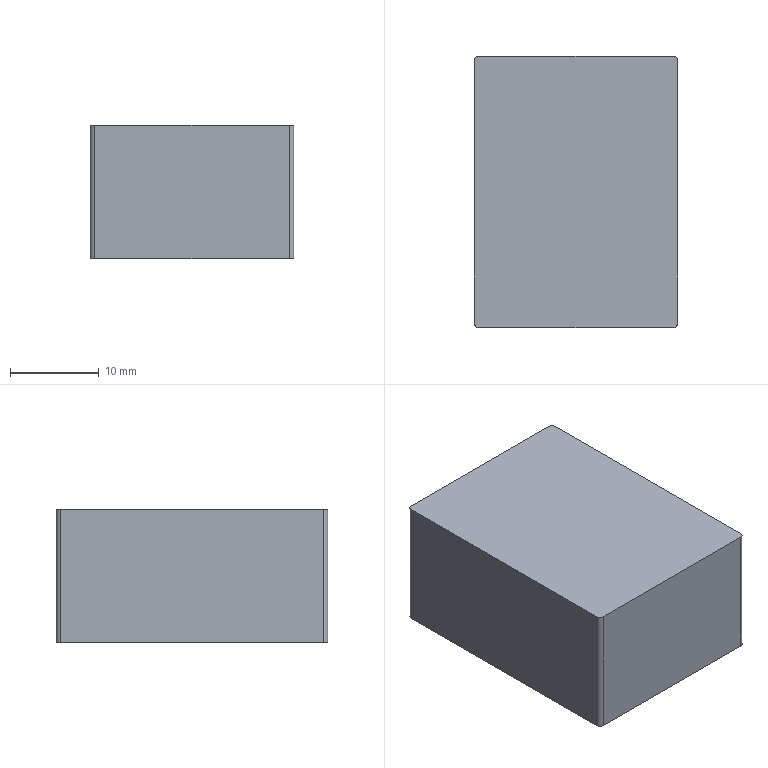Part | NX | features BREP 1 | 1 solid | 10 faces | box 22.892 x 30.505 x 15 mm | volume 10472 mm3 | plane 6 | cylinder 4 | commonest cylinder face diameters 1 x4
STEP:
#1=CARTESIAN_POINT('',(-10.946,15.253,-25.6));
#2=VERTEX_POINT('',#1);
#3=CARTESIAN_POINT('',(-11.446,14.753,-25.6));
#4=VERTEX_POINT('',#3);
#5=CARTESIAN_POINT('',(-10.946,14.753,-25.6));
#6=DIRECTION('',(0.,0.,1.));
#7=DIRECTION('',(1.,0.,0.));
#8=AXIS2_PLACEMENT_3D('',#5,#6,#7);
#9=CIRCLE('',#8,0.5);
#10=EDGE_CURVE('',#2,#4,#9,.T.);
#11=ORIENTED_EDGE('',*,*,#10,.F.);
#12=CARTESIAN_POINT('',(-10.946,15.253,-40.6));
#13=VERTEX_POINT('',#12);
#14=CARTESIAN_POINT('',(-10.946,15.253,-40.6));
#15=DIRECTION('',(0.,0.,1.));
#16=VECTOR('',#15,1000.);
#17=LINE('',#14,#16);
#18=EDGE_CURVE('',#13,#2,#17,.T.);
#19=ORIENTED_EDGE('',*,*,#18,.F.);
#20=CARTESIAN_POINT('',(-11.446,14.753,-40.6));
#21=VERTEX_POINT('',#20);
#22=CARTESIAN_POINT('',(-10.946,14.753,-40.6));
#23=DIRECTION('',(0.,0.,1.));
#24=DIRECTION('',(1.,0.,0.));
#25=AXIS2_PLACEMENT_3D('',#22,#23,#24);
#26=CIRCLE('',#25,0.5);
#27=EDGE_CURVE('',#13,#21,#26,.T.);
#28=ORIENTED_EDGE('',*,*,#27,.T.);
#29=CARTESIAN_POINT('',(-11.446,14.753,-40.6));
#30=DIRECTION('',(0.,0.,1.));
#31=VECTOR('',#30,1000.);
#32=LINE('',#29,#31);
#33=EDGE_CURVE('',#21,#4,#32,.T.);
#34=ORIENTED_EDGE('',*,*,#33,.T.);
#35=EDGE_LOOP('',(#11,#19,#28,#34));
#36=FACE_BOUND('',#35,.T.);
#37=CARTESIAN_POINT('',(-10.946,14.753,-40.6));
#38=DIRECTION('',(0.,0.,1.));
#39=DIRECTION('',(-1.,0.,0.));
#40=AXIS2_PLACEMENT_3D('',#37,#38,#39);
#41=CYLINDRICAL_SURFACE('',#40,0.5);
#42=ADVANCED_FACE('',(#36),#41,.T.);
#43=CARTESIAN_POINT('',(-11.446,-14.753,-25.6));
#44=VERTEX_POINT('',#43);
#45=CARTESIAN_POINT('',(-11.446,-14.753,-25.6));
#46=DIRECTION('',(0.,1.,0.));
#47=VECTOR('',#46,1000.);
#48=LINE('',#45,#47);
#49=EDGE_CURVE('',#44,#4,#48,.T.);
#50=ORIENTED_EDGE('',*,*,#49,.T.);
#51=ORIENTED_EDGE('',*,*,#33,.F.);
#52=CARTESIAN_POINT('',(-11.446,-14.753,-40.6));
#53=VERTEX_POINT('',#52);
#54=CARTESIAN_POINT('',(-11.446,-14.753,-40.6));
#55=DIRECTION('',(0.,1.,0.));
#56=VECTOR('',#55,1000.);
#57=LINE('',#54,#56);
#58=EDGE_CURVE('',#53,#21,#57,.T.);
#59=ORIENTED_EDGE('',*,*,#58,.F.);
#60=CARTESIAN_POINT('',(-11.446,-14.753,-40.6));
#61=DIRECTION('',(0.,0.,1.));
#62=VECTOR('',#61,1000.);
#63=LINE('',#60,#62);
#64=EDGE_CURVE('',#53,#44,#63,.T.);
#65=ORIENTED_EDGE('',*,*,#64,.T.);
#66=EDGE_LOOP('',(#50,#51,#59,#65));
#67=FACE_BOUND('',#66,.T.);
#68=CARTESIAN_POINT('',(-11.446,-14.753,-40.6));
#69=DIRECTION('',(1.,0.,0.));
#70=DIRECTION('',(0.,-1.,0.));
#71=AXIS2_PLACEMENT_3D('',#68,#69,#70);
#72=PLANE('',#71);
#73=ADVANCED_FACE('',(#67),#72,.F.);
#74=CARTESIAN_POINT('',(-10.946,-15.253,-25.6));
#75=VERTEX_POINT('',#74);
#76=CARTESIAN_POINT('',(-10.946,-14.753,-25.6));
#77=DIRECTION('',(0.,0.,1.));
#78=DIRECTION('',(1.,0.,0.));
#79=AXIS2_PLACEMENT_3D('',#76,#77,#78);
#80=CIRCLE('',#79,0.5);
#81=EDGE_CURVE('',#44,#75,#80,.T.);
#82=ORIENTED_EDGE('',*,*,#81,.F.);
#83=ORIENTED_EDGE('',*,*,#64,.F.);
#84=CARTESIAN_POINT('',(-10.946,-15.253,-40.6));
#85=VERTEX_POINT('',#84);
#86=CARTESIAN_POINT('',(-10.946,-14.753,-40.6));
#87=DIRECTION('',(0.,0.,1.));
#88=DIRECTION('',(1.,0.,0.));
#89=AXIS2_PLACEMENT_3D('',#86,#87,#88);
#90=CIRCLE('',#89,0.5);
#91=EDGE_CURVE('',#53,#85,#90,.T.);
#92=ORIENTED_EDGE('',*,*,#91,.T.);
#93=CARTESIAN_POINT('',(-10.946,-15.253,-40.6));
#94=DIRECTION('',(0.,0.,1.));
#95=VECTOR('',#94,1000.);
#96=LINE('',#93,#95);
#97=EDGE_CURVE('',#85,#75,#96,.T.);
#98=ORIENTED_EDGE('',*,*,#97,.T.);
#99=EDGE_LOOP('',(#82,#83,#92,#98));
#100=FACE_BOUND('',#99,.T.);
#101=CARTESIAN_POINT('',(-10.946,-14.753,-40.6));
#102=DIRECTION('',(0.,0.,1.));
#103=DIRECTION('',(-1.,0.,0.));
#104=AXIS2_PLACEMENT_3D('',#101,#102,#103);
#105=CYLINDRICAL_SURFACE('',#104,0.5);
#106=ADVANCED_FACE('',(#100),#105,.T.);
#107=CARTESIAN_POINT('',(10.946,-15.253,-25.6));
#108=VERTEX_POINT('',#107);
#109=CARTESIAN_POINT('',(10.946,-15.253,-25.6));
#110=DIRECTION('',(-1.,0.,0.));
#111=VECTOR('',#110,1000.);
#112=LINE('',#109,#111);
#113=EDGE_CURVE('',#108,#75,#112,.T.);
#114=ORIENTED_EDGE('',*,*,#113,.T.);
#115=ORIENTED_EDGE('',*,*,#97,.F.);
#116=CARTESIAN_POINT('',(10.946,-15.253,-40.6));
#117=VERTEX_POINT('',#116);
#118=CARTESIAN_POINT('',(10.946,-15.253,-40.6));
#119=DIRECTION('',(-1.,0.,0.));
#120=VECTOR('',#119,1000.);
#121=LINE('',#118,#120);
#122=EDGE_CURVE('',#117,#85,#121,.T.);
#123=ORIENTED_EDGE('',*,*,#122,.F.);
#124=CARTESIAN_POINT('',(10.946,-15.253,-40.6));
#125=DIRECTION('',(0.,0.,1.));
#126=VECTOR('',#125,1000.);
#127=LINE('',#124,#126);
#128=EDGE_CURVE('',#117,#108,#127,.T.);
#129=ORIENTED_EDGE('',*,*,#128,.T.);
#130=EDGE_LOOP('',(#114,#115,#123,#129));
#131=FACE_BOUND('',#130,.T.);
#132=CARTESIAN_POINT('',(10.946,-15.253,-40.6));
#133=DIRECTION('',(0.,1.,0.));
#134=DIRECTION('',(1.,0.,0.));
#135=AXIS2_PLACEMENT_3D('',#132,#133,#134);
#136=PLANE('',#135);
#137=ADVANCED_FACE('',(#131),#136,.F.);
#138=CARTESIAN_POINT('',(11.446,-14.753,-25.6));
#139=VERTEX_POINT('',#138);
#140=CARTESIAN_POINT('',(10.946,-14.753,-25.6));
#141=DIRECTION('',(0.,0.,1.));
#142=DIRECTION('',(1.,0.,0.));
#143=AXIS2_PLACEMENT_3D('',#140,#141,#142);
#144=CIRCLE('',#143,0.5);
#145=EDGE_CURVE('',#108,#139,#144,.T.);
#146=ORIENTED_EDGE('',*,*,#145,.F.);
#147=ORIENTED_EDGE('',*,*,#128,.F.);
#148=CARTESIAN_POINT('',(11.446,-14.753,-40.6));
#149=VERTEX_POINT('',#148);
#150=CARTESIAN_POINT('',(10.946,-14.753,-40.6));
#151=DIRECTION('',(0.,0.,1.));
#152=DIRECTION('',(1.,0.,0.));
#153=AXIS2_PLACEMENT_3D('',#150,#151,#152);
#154=CIRCLE('',#153,0.5);
#155=EDGE_CURVE('',#117,#149,#154,.T.);
#156=ORIENTED_EDGE('',*,*,#155,.T.);
#157=CARTESIAN_POINT('',(11.446,-14.753,-40.6));
#158=DIRECTION('',(0.,0.,1.));
#159=VECTOR('',#158,1000.);
#160=LINE('',#157,#159);
#161=EDGE_CURVE('',#149,#139,#160,.T.);
#162=ORIENTED_EDGE('',*,*,#161,.T.);
#163=EDGE_LOOP('',(#146,#147,#156,#162));
#164=FACE_BOUND('',#163,.T.);
#165=CARTESIAN_POINT('',(10.946,-14.753,-40.6));
#166=DIRECTION('',(0.,0.,1.));
#167=DIRECTION('',(-1.,0.,0.));
#168=AXIS2_PLACEMENT_3D('',#165,#166,#167);
#169=CYLINDRICAL_SURFACE('',#168,0.5);
#170=ADVANCED_FACE('',(#164),#169,.T.);
#171=CARTESIAN_POINT('',(11.446,14.753,-25.6));
#172=VERTEX_POINT('',#171);
#173=CARTESIAN_POINT('',(11.446,14.753,-25.6));
#174=DIRECTION('',(0.,-1.,0.));
#175=VECTOR('',#174,1000.);
#176=LINE('',#173,#175);
#177=EDGE_CURVE('',#172,#139,#176,.T.);
#178=ORIENTED_EDGE('',*,*,#177,.T.);
#179=ORIENTED_EDGE('',*,*,#161,.F.);
#180=CARTESIAN_POINT('',(11.446,14.753,-40.6));
#181=VERTEX_POINT('',#180);
#182=CARTESIAN_POINT('',(11.446,14.753,-40.6));
#183=DIRECTION('',(0.,-1.,0.));
#184=VECTOR('',#183,1000.);
#185=LINE('',#182,#184);
#186=EDGE_CURVE('',#181,#149,#185,.T.);
#187=ORIENTED_EDGE('',*,*,#186,.F.);
#188=CARTESIAN_POINT('',(11.446,14.753,-40.6));
#189=DIRECTION('',(0.,0.,1.));
#190=VECTOR('',#189,1000.);
#191=LINE('',#188,#190);
#192=EDGE_CURVE('',#181,#172,#191,.T.);
#193=ORIENTED_EDGE('',*,*,#192,.T.);
#194=EDGE_LOOP('',(#178,#179,#187,#193));
#195=FACE_BOUND('',#194,.T.);
#196=CARTESIAN_POINT('',(11.446,14.753,-40.6));
#197=DIRECTION('',(-1.,0.,0.));
#198=DIRECTION('',(0.,1.,0.));
#199=AXIS2_PLACEMENT_3D('',#196,#197,#198);
#200=PLANE('',#199);
#201=ADVANCED_FACE('',(#195),#200,.F.);
#202=CARTESIAN_POINT('',(10.946,15.253,-25.6));
#203=VERTEX_POINT('',#202);
#204=CARTESIAN_POINT('',(10.946,14.753,-25.6));
#205=DIRECTION('',(0.,0.,1.));
#206=DIRECTION('',(1.,0.,0.));
#207=AXIS2_PLACEMENT_3D('',#204,#205,#206);
#208=CIRCLE('',#207,0.5);
#209=EDGE_CURVE('',#172,#203,#208,.T.);
#210=ORIENTED_EDGE('',*,*,#209,.F.);
#211=ORIENTED_EDGE('',*,*,#192,.F.);
#212=CARTESIAN_POINT('',(10.946,15.253,-40.6));
#213=VERTEX_POINT('',#212);
#214=CARTESIAN_POINT('',(10.946,14.753,-40.6));
#215=DIRECTION('',(0.,0.,1.));
#216=DIRECTION('',(1.,0.,0.));
#217=AXIS2_PLACEMENT_3D('',#214,#215,#216);
#218=CIRCLE('',#217,0.5);
#219=EDGE_CURVE('',#181,#213,#218,.T.);
#220=ORIENTED_EDGE('',*,*,#219,.T.);
#221=CARTESIAN_POINT('',(10.946,15.253,-40.6));
#222=DIRECTION('',(0.,0.,1.));
#223=VECTOR('',#222,1000.);
#224=LINE('',#221,#223);
#225=EDGE_CURVE('',#213,#203,#224,.T.);
#226=ORIENTED_EDGE('',*,*,#225,.T.);
#227=EDGE_LOOP('',(#210,#211,#220,#226));
#228=FACE_BOUND('',#227,.T.);
#229=CARTESIAN_POINT('',(10.946,14.753,-40.6));
#230=DIRECTION('',(0.,0.,1.));
#231=DIRECTION('',(-1.,0.,0.));
#232=AXIS2_PLACEMENT_3D('',#229,#230,#231);
#233=CYLINDRICAL_SURFACE('',#232,0.5);
#234=ADVANCED_FACE('',(#228),#233,.T.);
#235=CARTESIAN_POINT('',(-10.946,15.253,-25.6));
#236=DIRECTION('',(1.,0.,0.));
#237=VECTOR('',#236,1000.);
#238=LINE('',#235,#237);
#239=EDGE_CURVE('',#2,#203,#238,.T.);
#240=ORIENTED_EDGE('',*,*,#239,.T.);
#241=ORIENTED_EDGE('',*,*,#225,.F.);
#242=CARTESIAN_POINT('',(-10.946,15.253,-40.6));
#243=DIRECTION('',(1.,0.,0.));
#244=VECTOR('',#243,1000.);
#245=LINE('',#242,#244);
#246=EDGE_CURVE('',#13,#213,#245,.T.);
#247=ORIENTED_EDGE('',*,*,#246,.F.);
#248=ORIENTED_EDGE('',*,*,#18,.T.);
#249=EDGE_LOOP('',(#240,#241,#247,#248));
#250=FACE_BOUND('',#249,.T.);
#251=CARTESIAN_POINT('',(-10.946,15.253,-40.6));
#252=DIRECTION('',(0.,-1.,0.));
#253=DIRECTION('',(0.,0.,1.));
#254=AXIS2_PLACEMENT_3D('',#251,#252,#253);
#255=PLANE('',#254);
#256=ADVANCED_FACE('',(#250),#255,.F.);
#257=ORIENTED_EDGE('',*,*,#27,.F.);
#258=ORIENTED_EDGE('',*,*,#246,.T.);
#259=ORIENTED_EDGE('',*,*,#219,.F.);
#260=ORIENTED_EDGE('',*,*,#186,.T.);
#261=ORIENTED_EDGE('',*,*,#155,.F.);
#262=ORIENTED_EDGE('',*,*,#122,.T.);
#263=ORIENTED_EDGE('',*,*,#91,.F.);
#264=ORIENTED_EDGE('',*,*,#58,.T.);
#265=EDGE_LOOP('',(#257,#258,#259,#260,#261,#262,#263,#264));
#266=FACE_BOUND('',#265,.T.);
#267=CARTESIAN_POINT('',(-10.946,14.753,-40.6));
#268=DIRECTION('',(0.,0.,1.));
#269=DIRECTION('',(-1.,0.,0.));
#270=AXIS2_PLACEMENT_3D('',#267,#268,#269);
#271=PLANE('',#270);
#272=ADVANCED_FACE('',(#266),#271,.F.);
#273=ORIENTED_EDGE('',*,*,#10,.T.);
#274=ORIENTED_EDGE('',*,*,#49,.F.);
#275=ORIENTED_EDGE('',*,*,#81,.T.);
#276=ORIENTED_EDGE('',*,*,#113,.F.);
#277=ORIENTED_EDGE('',*,*,#145,.T.);
#278=ORIENTED_EDGE('',*,*,#177,.F.);
#279=ORIENTED_EDGE('',*,*,#209,.T.);
#280=ORIENTED_EDGE('',*,*,#239,.F.);
#281=EDGE_LOOP('',(#273,#274,#275,#276,#277,#278,#279,#280));
#282=FACE_BOUND('',#281,.T.);
#283=CARTESIAN_POINT('',(-10.946,14.753,-25.6));
#284=DIRECTION('',(0.,0.,1.));
#285=DIRECTION('',(-1.,0.,0.));
#286=AXIS2_PLACEMENT_3D('',#283,#284,#285);
#287=PLANE('',#286);
#288=ADVANCED_FACE('',(#282),#287,.T.);
#289=CLOSED_SHELL('',(#42,#73,#106,#137,#170,#201,#234,#256,#272,#288));
#290=MANIFOLD_SOLID_BREP('',#289);
#291=(LENGTH_UNIT()NAMED_UNIT(*)SI_UNIT(.MILLI.,.METRE.));
#292=UNCERTAINTY_MEASURE_WITH_UNIT(LENGTH_MEASURE(0.00001),#291,'','');
#293=(NAMED_UNIT(*)PLANE_ANGLE_UNIT()SI_UNIT($,.RADIAN.));
#294=(NAMED_UNIT(*)SI_UNIT($,.STERADIAN.)SOLID_ANGLE_UNIT());
#295=(GEOMETRIC_REPRESENTATION_CONTEXT(3)GLOBAL_UNCERTAINTY_ASSIGNED_CONTEXT((#292))GLOBAL_UNIT_ASSIGNED_CONTEXT((#291,#293,#294))REPRESENTATION_CONTEXT('',''));
#296=ADVANCED_BREP_SHAPE_REPRESENTATION('',(#290),#295);